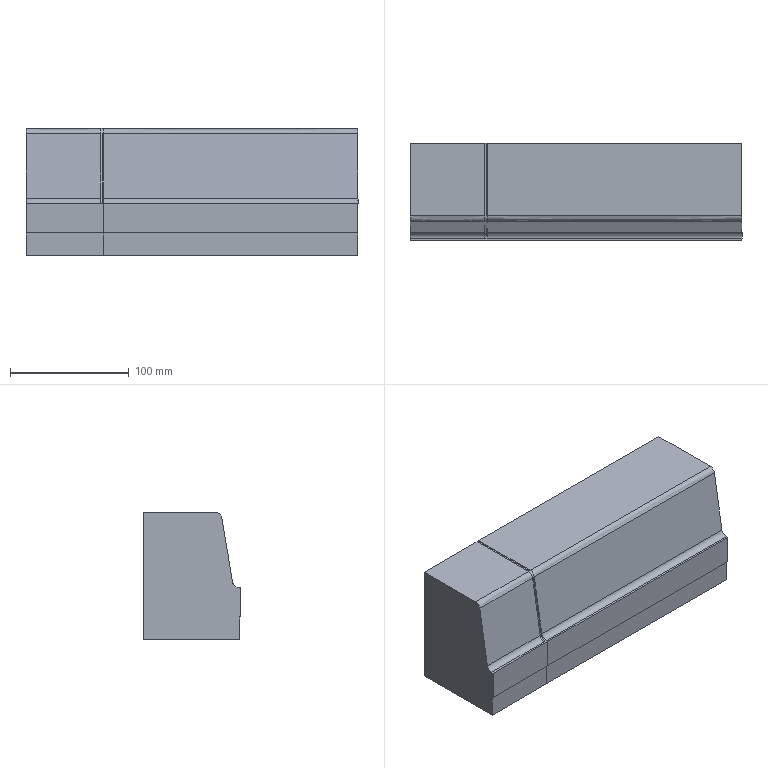Part | NX | features solid 2 | 1 solid | 36 faces | box 280 x 82.346 x 107.138 mm | volume 2225782 mm3 | spline 13 | plane 10 | cylinder 9 | cone 3 | sphere 1 | commonest cylinder face diameters 10 x3 12 x3 20 x2 14 x1